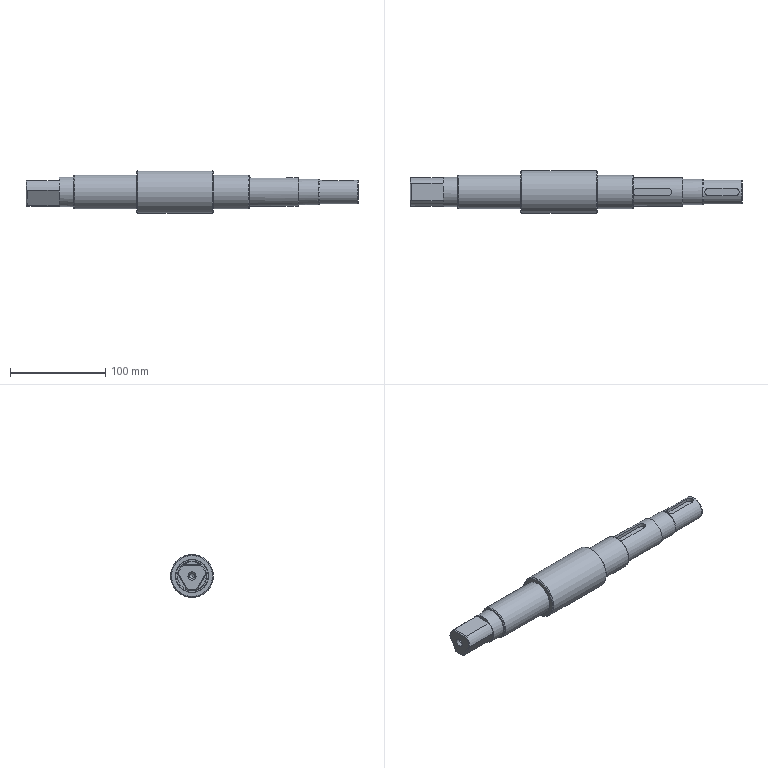CAM job | NX | 3+2 milling, drilling | part box 348.4 x 45 x 45 mm
Tools:
number,name,description,diameter,corner_radius,flute_length,length,flutes
1,ZXZ,Milling Tool-5 Parameters,6.0,0.0,50.0,75.0,2
15,5.0ZT,Drilling Tool,5.0,0.0,35.0,50.0,2
12,D12,Milling Tool-5 Parameters,12.0,0.0,50.0,75.0,2
7,D6A45,Milling Tool-5 Parameters,6.0,0.0,50.0,75.0,2
14,M6,Milling Tool-5 Parameters,5.0,0.0,30.0,30.0,4
6,D6,Milling Tool-5 Parameters,6.0,0.0,50.0,75.0,2
4,D4,Milling Tool-5 Parameters,4.0,0.0,50.0,75.0,2
Operations:
program,operation,operation_type,tool,method,geometry_group,spindle_rpm,surface_speed,feed_per_tooth,feed_cut,feed_plunge,cut_length_mm,path_length_mm,cut_time_min,machine_time_min
1,DRILLING,Operation,ZXZ,METHOD,A,5000.0,94.0,0.025,250.0,0.0,4.0,68.0,0.016,0.0224
1,DRILLING_COPY_COPY_1,Operation,5.0ZT,METHOD,A,2000.0,56.0,0.0375,150.0,0.0,27.502,115.004,0.1833,0.1921
1,DRILLING_COPY_2_COPY_COPY_1_COPY_COPY,Operation,M6,METHOD,A,200.0,3.0,0.0013,1.0,0.0,26.0,112.0,26.0,26.009
1,ZLEVEL_PROFILE,ZLevelMilling,D12,METHOD,A,3000.0,94.0,0.3667,2200.0,1000.0,22578.572,22667.372,10.33,10.338
1,PLANAR_MILL_COPY_COPY,PlanarMilling,D6A45,METHOD,A,7500.0,141.0,0.0833,1250.0,100.0,325.849,384.849,0.2607,0.2666
1,PLANAR_MILL_COPY_COPY_COPY,PlanarMilling,D6A45,METHOD,A,7500.0,141.0,0.0833,1250.0,100.0,17.17,74.17,0.0137,0.0194
1,刀补12,ZLevelMilling,D12,METHOD,A,5000.0,157.0,0.125,1250.0,100.0,4861.96,8220.635,3.89,4.225
2,刀补6,ZLevelMilling,D6,METHOD,B,4500.0,84.0,0.1833,1650.0,1000.0,4295.832,4370.798,2.612,2.619
2,刀补6_COPY,ZLevelMilling,D6,METHOD,B,4500.0,84.0,0.1833,1650.0,1000.0,2878.409,2959.875,1.753,1.761
3,刀补4,ZLevelMilling,D4,METHOD,C,4500.0,84.0,0.1833,1650.0,1000.0,1441.895,1518.903,0.8819,0.8896